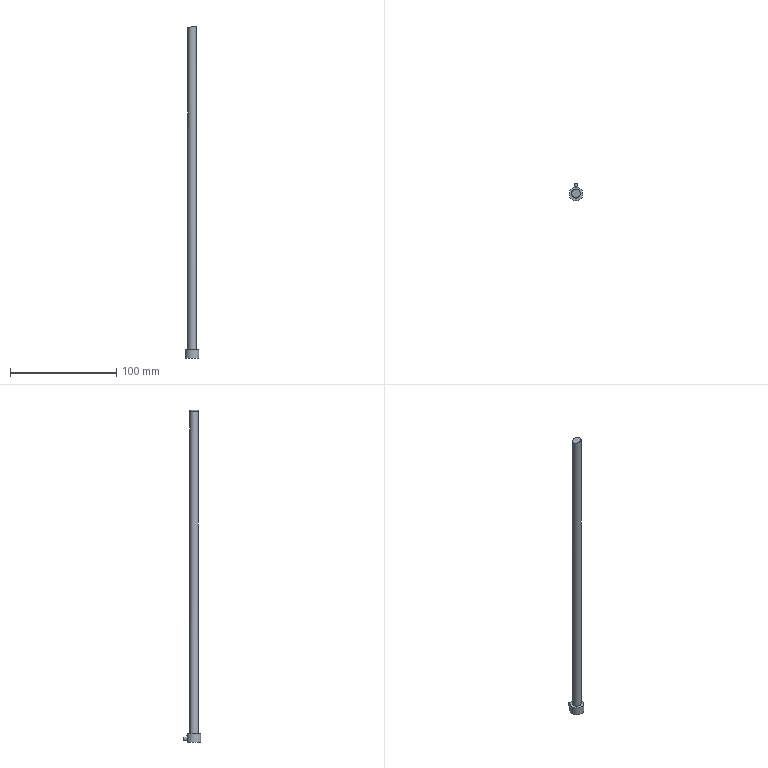Part | STEP file | E108-03-320 | 1 solid | 8 faces | box 13 x 16.5 x 312.703 mm | volume 16360 mm3 | cylinder 3 | plane 3 | spline 1 | cone 1 | commonest cylinder face diameters 3 x1 8 x1 13 x1
STEP:
#1=CARTESIAN_POINT('',(0.,0.,0.));
#2=DIRECTION('',(0.,0.,1.));
#3=DIRECTION('',(1.,0.,0.));
#4=AXIS2_PLACEMENT_3D('',#1,#2,#3);
#5=CARTESIAN_POINT('',(-3.956,0.5934,310.968));
#6=VERTEX_POINT('',#5);
#7=CARTESIAN_POINT('',(-3.956,0.5934,310.968));
#8=CARTESIAN_POINT('',(-4.021,0.1589,310.969));
#9=CARTESIAN_POINT('',(-4.013,-0.2925,310.988));
#10=CARTESIAN_POINT('',(-3.934,-0.7232,311.022));
#11=CARTESIAN_POINT('',(-3.855,-1.154,311.057));
#12=CARTESIAN_POINT('',(-3.702,-1.575,311.108));
#13=CARTESIAN_POINT('',(-3.49,-1.955,311.17));
#14=CARTESIAN_POINT('',(-3.275,-2.338,311.234));
#15=CARTESIAN_POINT('',(-2.993,-2.689,311.311));
#16=CARTESIAN_POINT('',(-2.668,-2.98,311.395));
#17=CARTESIAN_POINT('',(-2.335,-3.279,311.481));
#18=CARTESIAN_POINT('',(-1.947,-3.523,311.576));
#19=CARTESIAN_POINT('',(-1.535,-3.694,311.673));
#20=CARTESIAN_POINT('',(-1.116,-3.868,311.772));
#21=CARTESIAN_POINT('',(-0.6599,-3.971,311.874));
#22=CARTESIAN_POINT('',(-0.2055,-3.995,311.972));
#23=CARTESIAN_POINT('',(0.2524,-4.018,312.071));
#24=CARTESIAN_POINT('',(0.7217,-3.961,312.168));
#25=CARTESIAN_POINT('',(1.163,-3.827,312.255));
#26=CARTESIAN_POINT('',(1.6,-3.694,312.342));
#27=CARTESIAN_POINT('',(2.022,-3.482,312.42));
#28=CARTESIAN_POINT('',(2.391,-3.206,312.485));
#29=CARTESIAN_POINT('',(2.753,-2.936,312.549));
#30=CARTESIAN_POINT('',(3.075,-2.598,312.601));
#31=CARTESIAN_POINT('',(3.328,-2.22,312.637));
#32=CARTESIAN_POINT('',(3.575,-1.849,312.673));
#33=CARTESIAN_POINT('',(3.762,-1.43,312.695));
#34=CARTESIAN_POINT('',(3.874,-0.9979,312.701));
#35=CARTESIAN_POINT('',(3.983,-0.5714,312.707));
#36=CARTESIAN_POINT('',(4.022,-0.1202,312.698));
#37=CARTESIAN_POINT('',(3.987,0.3182,312.675));
#38=CARTESIAN_POINT('',(3.952,0.7555,312.652));
#39=CARTESIAN_POINT('',(3.843,1.192,312.614));
#40=CARTESIAN_POINT('',(3.669,1.593,312.565));
#41=CARTESIAN_POINT('',(3.494,1.997,312.516));
#42=CARTESIAN_POINT('',(3.248,2.375,312.453));
#43=CARTESIAN_POINT('',(2.953,2.698,312.381));
#44=CARTESIAN_POINT('',(2.653,3.027,312.309));
#45=CARTESIAN_POINT('',(2.293,3.307,312.225));
#46=CARTESIAN_POINT('',(1.904,3.518,312.137));
#47=CARTESIAN_POINT('',(1.508,3.732,312.048));
#48=CARTESIAN_POINT('',(1.069,3.881,311.951));
#49=CARTESIAN_POINT('',(0.6254,3.951,311.854));
#50=CARTESIAN_POINT('',(0.1749,4.022,311.757));
#51=CARTESIAN_POINT('',(-0.2942,4.015,311.656));
#52=CARTESIAN_POINT('',(-0.7432,3.93,311.562));
#53=CARTESIAN_POINT('',(-1.193,3.845,311.467));
#54=CARTESIAN_POINT('',(-1.636,3.679,311.376));
#55=CARTESIAN_POINT('',(-2.033,3.445,311.297));
#56=CARTESIAN_POINT('',(-2.425,3.213,311.218));
#57=CARTESIAN_POINT('',(-2.784,2.908,311.149));
#58=CARTESIAN_POINT('',(-3.078,2.555,311.095));
#59=CARTESIAN_POINT('',(-3.364,2.21,311.043));
#60=CARTESIAN_POINT('',(-3.596,1.809,311.005));
#61=CARTESIAN_POINT('',(-3.753,1.385,310.985));
#62=CARTESIAN_POINT('',(-3.847,1.13,310.973));
#63=CARTESIAN_POINT('',(-3.915,0.8629,310.967));
#64=CARTESIAN_POINT('',(-3.956,0.5934,310.968));
#65=B_SPLINE_CURVE_WITH_KNOTS('',3,(#7,#8,#9,#10,#11,#12,#13,#14,#15,#16,#17,#18,#19,#20,#21,#22,#23,#24,#25,#26,#27,#28,#29,#30,#31,#32,#33,#34,#35,#36,#37,#38,#39,#40,#41,#42,#43,#44,#45,#46,#47,#48,#49,#50,#51,#52,#53,#54,#55,#56,#57,#58,#59,#60,#61,#62,#63,#64),.UNSPECIFIED.,.T.,.F.,(1,3,3,3,3,3,3,3,3,3,3,3,3,3,3,3,3,3,3,3,3,1),(-0.03202,0.,0.05208,0.1041,0.1568,0.2108,0.266,0.3216,0.3768,0.431,0.4839,0.5361,0.5882,0.6407,0.6942,0.7487,0.804,0.8595,0.9144,0.968,1.,1.052),.UNSPECIFIED.);
#66=CARTESIAN_POINT('',(0.,0.,108.));
#67=DIRECTION('',(0.,0.,-1.));
#68=DIRECTION('',(-1.,0.,0.));
#69=AXIS2_PLACEMENT_3D('',#66,#67,#68);
#70=CYLINDRICAL_SURFACE('',#69,4.);
#71=CARTESIAN_POINT('',(6.432,-202.968));
#72=CARTESIAN_POINT('',(6.408,-202.968));
#73=CARTESIAN_POINT('',(6.36,-202.971));
#74=CARTESIAN_POINT('',(6.288,-202.979));
#75=CARTESIAN_POINT('',(6.215,-202.992));
#76=CARTESIAN_POINT('',(6.143,-203.009));
#77=CARTESIAN_POINT('',(6.072,-203.031));
#78=CARTESIAN_POINT('',(6.,-203.058));
#79=CARTESIAN_POINT('',(5.928,-203.089));
#80=CARTESIAN_POINT('',(5.856,-203.124));
#81=CARTESIAN_POINT('',(5.784,-203.163));
#82=CARTESIAN_POINT('',(5.713,-203.205));
#83=CARTESIAN_POINT('',(5.642,-203.251));
#84=CARTESIAN_POINT('',(5.57,-203.3));
#85=CARTESIAN_POINT('',(5.499,-203.352));
#86=CARTESIAN_POINT('',(5.428,-203.405));
#87=CARTESIAN_POINT('',(5.358,-203.461));
#88=CARTESIAN_POINT('',(5.287,-203.519));
#89=CARTESIAN_POINT('',(5.216,-203.579));
#90=CARTESIAN_POINT('',(5.145,-203.639));
#91=CARTESIAN_POINT('',(5.075,-203.7));
#92=CARTESIAN_POINT('',(5.004,-203.762));
#93=CARTESIAN_POINT('',(4.934,-203.824));
#94=CARTESIAN_POINT('',(4.863,-203.886));
#95=CARTESIAN_POINT('',(4.792,-203.948));
#96=CARTESIAN_POINT('',(4.722,-204.008));
#97=CARTESIAN_POINT('',(4.651,-204.068));
#98=CARTESIAN_POINT('',(4.581,-204.127));
#99=CARTESIAN_POINT('',(4.51,-204.184));
#100=CARTESIAN_POINT('',(4.439,-204.239));
#101=CARTESIAN_POINT('',(4.368,-204.292));
#102=CARTESIAN_POINT('',(4.297,-204.343));
#103=CARTESIAN_POINT('',(4.226,-204.391));
#104=CARTESIAN_POINT('',(4.154,-204.437));
#105=CARTESIAN_POINT('',(4.083,-204.479));
#106=CARTESIAN_POINT('',(4.012,-204.518));
#107=CARTESIAN_POINT('',(3.94,-204.554));
#108=CARTESIAN_POINT('',(3.868,-204.587));
#109=CARTESIAN_POINT('',(3.796,-204.615));
#110=CARTESIAN_POINT('',(3.724,-204.64));
#111=CARTESIAN_POINT('',(3.653,-204.661));
#112=CARTESIAN_POINT('',(3.58,-204.677));
#113=CARTESIAN_POINT('',(3.508,-204.69));
#114=CARTESIAN_POINT('',(3.436,-204.699));
#115=CARTESIAN_POINT('',(3.364,-204.703));
#116=CARTESIAN_POINT('',(3.292,-204.703));
#117=CARTESIAN_POINT('',(3.219,-204.699));
#118=CARTESIAN_POINT('',(3.147,-204.69));
#119=CARTESIAN_POINT('',(3.075,-204.678));
#120=CARTESIAN_POINT('',(3.003,-204.662));
#121=CARTESIAN_POINT('',(2.931,-204.641));
#122=CARTESIAN_POINT('',(2.859,-204.617));
#123=CARTESIAN_POINT('',(2.787,-204.589));
#124=CARTESIAN_POINT('',(2.715,-204.558));
#125=CARTESIAN_POINT('',(2.643,-204.523));
#126=CARTESIAN_POINT('',(2.572,-204.485));
#127=CARTESIAN_POINT('',(2.5,-204.443));
#128=CARTESIAN_POINT('',(2.429,-204.399));
#129=CARTESIAN_POINT('',(2.358,-204.353));
#130=CARTESIAN_POINT('',(2.286,-204.303));
#131=CARTESIAN_POINT('',(2.215,-204.252));
#132=CARTESIAN_POINT('',(2.144,-204.198));
#133=CARTESIAN_POINT('',(2.073,-204.143));
#134=CARTESIAN_POINT('',(2.003,-204.086));
#135=CARTESIAN_POINT('',(1.932,-204.028));
#136=CARTESIAN_POINT('',(1.861,-203.968));
#137=CARTESIAN_POINT('',(1.79,-203.908));
#138=CARTESIAN_POINT('',(1.72,-203.848));
#139=CARTESIAN_POINT('',(1.649,-203.787));
#140=CARTESIAN_POINT('',(1.579,-203.726));
#141=CARTESIAN_POINT('',(1.508,-203.666));
#142=CARTESIAN_POINT('',(1.437,-203.606));
#143=CARTESIAN_POINT('',(1.367,-203.548));
#144=CARTESIAN_POINT('',(1.296,-203.49));
#145=CARTESIAN_POINT('',(1.225,-203.434));
#146=CARTESIAN_POINT('',(1.154,-203.38));
#147=CARTESIAN_POINT('',(1.083,-203.328));
#148=CARTESIAN_POINT('',(1.012,-203.279));
#149=CARTESIAN_POINT('',(0.941,-203.232));
#150=CARTESIAN_POINT('',(0.8695,-203.188));
#151=CARTESIAN_POINT('',(0.7978,-203.148));
#152=CARTESIAN_POINT('',(0.7262,-203.111));
#153=CARTESIAN_POINT('',(0.6549,-203.077));
#154=CARTESIAN_POINT('',(0.583,-203.048));
#155=CARTESIAN_POINT('',(0.5109,-203.023));
#156=CARTESIAN_POINT('',(0.4386,-203.003));
#157=CARTESIAN_POINT('',(0.3668,-202.987));
#158=CARTESIAN_POINT('',(0.2943,-202.975));
#159=CARTESIAN_POINT('',(0.2215,-202.969));
#160=CARTESIAN_POINT('',(0.1731,-202.968));
#161=CARTESIAN_POINT('',(0.1489,-202.968));
#162=B_SPLINE_CURVE_WITH_KNOTS('',3,(#71,#72,#73,#74,#75,#76,#77,#78,#79,#80,#81,#82,#83,#84,#85,#86,#87,#88,#89,#90,#91,#92,#93,#94,#95,#96,#97,#98,#99,#100,#101,#102,#103,#104,#105,#106,#107,#108,#109,#110,#111,#112,#113,#114,#115,#116,#117,#118,#119,#120,#121,#122,#123,#124,#125,#126,#127,#128,#129,#130,#131,#132,#133,#134,#135,#136,#137,#138,#139,#140,#141,#142,#143,#144,#145,#146,#147,#148,#149,#150,#151,#152,#153,#154,#155,#156,#157,#158,#159,#160,#161),.UNSPECIFIED.,.F.,.F.,(4,1,1,1,1,1,1,1,1,1,1,1,1,1,1,1,1,1,1,1,1,1,1,1,1,1,1,1,1,1,1,1,1,1,1,1,1,1,1,1,1,1,1,1,1,1,1,1,1,1,1,1,1,1,1,1,1,1,1,1,1,1,1,1,1,1,1,1,1,1,1,1,1,1,1,1,1,1,1,1,1,1,1,1,1,1,1,1,4),(0.,0.01136,0.02273,0.03409,0.04545,0.05682,0.06818,0.07955,0.09091,0.1023,0.1136,0.125,0.1364,0.1477,0.1591,0.1705,0.1818,0.1932,0.2045,0.2159,0.2273,0.2386,0.25,0.2614,0.2727,0.2841,0.2955,0.3068,0.3182,0.3295,0.3409,0.3523,0.3636,0.375,0.3864,0.3977,0.4091,0.4205,0.4318,0.4432,0.4545,0.4659,0.4773,0.4886,0.5,0.5114,0.5227,0.5341,0.5455,0.5568,0.5682,0.5795,0.5909,0.6023,0.6136,0.625,0.6364,0.6477,0.6591,0.6705,0.6818,0.6932,0.7045,0.7159,0.7273,0.7386,0.75,0.7614,0.7727,0.7841,0.7955,0.8068,0.8182,0.8295,0.8409,0.8523,0.8636,0.875,0.8864,0.8977,0.9091,0.9205,0.9318,0.9432,0.9545,0.9659,0.9773,0.9886,1.),.QUASI_UNIFORM_KNOTS.);
#163=(GEOMETRIC_REPRESENTATION_CONTEXT(2)PARAMETRIC_REPRESENTATION_CONTEXT()REPRESENTATION_CONTEXT('',''));
#164=DEFINITIONAL_REPRESENTATION('',(#162),#163);
#165=PCURVE('',#70,#164);
#166=CARTESIAN_POINT('',(-4.984,-7.122,311.018));
#167=CARTESIAN_POINT('',(-1.231,-7.119,311.896));
#168=CARTESIAN_POINT('',(2.537,-7.117,312.689));
#169=CARTESIAN_POINT('',(6.321,-7.115,313.394));
#170=CARTESIAN_POINT('',(-4.925,-2.039,310.842));
#171=CARTESIAN_POINT('',(-1.173,-2.037,311.72));
#172=CARTESIAN_POINT('',(2.593,-2.035,312.514));
#173=CARTESIAN_POINT('',(6.376,-2.033,313.219));
#174=CARTESIAN_POINT('',(-4.869,3.043,310.664));
#175=CARTESIAN_POINT('',(-1.118,3.045,311.543));
#176=CARTESIAN_POINT('',(2.646,3.047,312.337));
#177=CARTESIAN_POINT('',(6.428,3.049,313.043));
#178=CARTESIAN_POINT('',(-4.816,8.125,310.485));
#179=CARTESIAN_POINT('',(-1.066,8.127,311.364));
#180=CARTESIAN_POINT('',(2.697,8.129,312.159));
#181=CARTESIAN_POINT('',(6.478,8.131,312.866));
#182=B_SPLINE_SURFACE_WITH_KNOTS('',3,3,((#166,#167,#168,#169),(#170,#171,#172,#173),(#174,#175,#176,#177),(#178,#179,#180,#181)),.UNSPECIFIED.,.F.,.F.,.F.,(4,4),(4,4),(0.,1.),(0.,1.),.PIECEWISE_BEZIER_KNOTS.);
#183=CARTESIAN_POINT('',(0.506,0.0836));
#184=CARTESIAN_POINT('',(0.4998,0.08243));
#185=CARTESIAN_POINT('',(0.4872,0.08071));
#186=CARTESIAN_POINT('',(0.4683,0.07997));
#187=CARTESIAN_POINT('',(0.4493,0.08106));
#188=CARTESIAN_POINT('',(0.4304,0.08398));
#189=CARTESIAN_POINT('',(0.4119,0.0887));
#190=CARTESIAN_POINT('',(0.3936,0.09527));
#191=CARTESIAN_POINT('',(0.3756,0.1036));
#192=CARTESIAN_POINT('',(0.3582,0.1136));
#193=CARTESIAN_POINT('',(0.3414,0.1252));
#194=CARTESIAN_POINT('',(0.3253,0.1383));
#195=CARTESIAN_POINT('',(0.3099,0.153));
#196=CARTESIAN_POINT('',(0.2953,0.1691));
#197=CARTESIAN_POINT('',(0.2816,0.1865));
#198=CARTESIAN_POINT('',(0.2689,0.205));
#199=CARTESIAN_POINT('',(0.2572,0.2248));
#200=CARTESIAN_POINT('',(0.2465,0.2456));
#201=CARTESIAN_POINT('',(0.237,0.2673));
#202=CARTESIAN_POINT('',(0.2286,0.2898));
#203=CARTESIAN_POINT('',(0.2214,0.3128));
#204=CARTESIAN_POINT('',(0.2155,0.3366));
#205=CARTESIAN_POINT('',(0.2108,0.3609));
#206=CARTESIAN_POINT('',(0.2073,0.3856));
#207=CARTESIAN_POINT('',(0.2052,0.4105));
#208=CARTESIAN_POINT('',(0.2043,0.4353));
#209=CARTESIAN_POINT('',(0.2048,0.4604));
#210=CARTESIAN_POINT('',(0.2066,0.4853));
#211=CARTESIAN_POINT('',(0.2097,0.5101));
#212=CARTESIAN_POINT('',(0.214,0.5344));
#213=CARTESIAN_POINT('',(0.2197,0.5581));
#214=CARTESIAN_POINT('',(0.2266,0.5814));
#215=CARTESIAN_POINT('',(0.2348,0.604));
#216=CARTESIAN_POINT('',(0.2441,0.6257));
#217=CARTESIAN_POINT('',(0.2545,0.6465));
#218=CARTESIAN_POINT('',(0.2661,0.6661));
#219=CARTESIAN_POINT('',(0.2787,0.6847));
#220=CARTESIAN_POINT('',(0.2924,0.7021));
#221=CARTESIAN_POINT('',(0.3069,0.7181));
#222=CARTESIAN_POINT('',(0.3222,0.7326));
#223=CARTESIAN_POINT('',(0.3384,0.7456));
#224=CARTESIAN_POINT('',(0.3552,0.757));
#225=CARTESIAN_POINT('',(0.3727,0.7668));
#226=CARTESIAN_POINT('',(0.3906,0.7748));
#227=CARTESIAN_POINT('',(0.4089,0.7811));
#228=CARTESIAN_POINT('',(0.4275,0.7855));
#229=CARTESIAN_POINT('',(0.4464,0.7881));
#230=CARTESIAN_POINT('',(0.4654,0.7889));
#231=CARTESIAN_POINT('',(0.4843,0.7879));
#232=CARTESIAN_POINT('',(0.503,0.785));
#233=CARTESIAN_POINT('',(0.5217,0.7803));
#234=CARTESIAN_POINT('',(0.5401,0.7738));
#235=CARTESIAN_POINT('',(0.558,0.7656));
#236=CARTESIAN_POINT('',(0.5754,0.7557));
#237=CARTESIAN_POINT('',(0.5922,0.7442));
#238=CARTESIAN_POINT('',(0.6084,0.731));
#239=CARTESIAN_POINT('',(0.6239,0.7164));
#240=CARTESIAN_POINT('',(0.6386,0.7004));
#241=CARTESIAN_POINT('',(0.6522,0.6831));
#242=CARTESIAN_POINT('',(0.665,0.6645));
#243=CARTESIAN_POINT('',(0.6767,0.6447));
#244=CARTESIAN_POINT('',(0.6874,0.6239));
#245=CARTESIAN_POINT('',(0.697,0.6023));
#246=CARTESIAN_POINT('',(0.7053,0.5799));
#247=CARTESIAN_POINT('',(0.7125,0.5566));
#248=CARTESIAN_POINT('',(0.7184,0.5328));
#249=CARTESIAN_POINT('',(0.7232,0.5084));
#250=CARTESIAN_POINT('',(0.7266,0.4839));
#251=CARTESIAN_POINT('',(0.7287,0.459));
#252=CARTESIAN_POINT('',(0.7295,0.434));
#253=CARTESIAN_POINT('',(0.729,0.4089));
#254=CARTESIAN_POINT('',(0.7272,0.384));
#255=CARTESIAN_POINT('',(0.7241,0.3594));
#256=CARTESIAN_POINT('',(0.7197,0.3351));
#257=CARTESIAN_POINT('',(0.714,0.3112));
#258=CARTESIAN_POINT('',(0.7071,0.2879));
#259=CARTESIAN_POINT('',(0.6989,0.2653));
#260=CARTESIAN_POINT('',(0.6897,0.2437));
#261=CARTESIAN_POINT('',(0.6792,0.2229));
#262=CARTESIAN_POINT('',(0.6676,0.2031));
#263=CARTESIAN_POINT('',(0.655,0.1844));
#264=CARTESIAN_POINT('',(0.6414,0.167));
#265=CARTESIAN_POINT('',(0.627,0.1511));
#266=CARTESIAN_POINT('',(0.6116,0.1365));
#267=CARTESIAN_POINT('',(0.5954,0.1235));
#268=CARTESIAN_POINT('',(0.5786,0.112));
#269=CARTESIAN_POINT('',(0.5612,0.1022));
#270=CARTESIAN_POINT('',(0.5432,0.09409));
#271=CARTESIAN_POINT('',(0.5248,0.08777));
#272=CARTESIAN_POINT('',(0.5123,0.08478));
#273=CARTESIAN_POINT('',(0.506,0.0836));
#274=B_SPLINE_CURVE_WITH_KNOTS('',3,(#183,#184,#185,#186,#187,#188,#189,#190,#191,#192,#193,#194,#195,#196,#197,#198,#199,#200,#201,#202,#203,#204,#205,#206,#207,#208,#209,#210,#211,#212,#213,#214,#215,#216,#217,#218,#219,#220,#221,#222,#223,#224,#225,#226,#227,#228,#229,#230,#231,#232,#233,#234,#235,#236,#237,#238,#239,#240,#241,#242,#243,#244,#245,#246,#247,#248,#249,#250,#251,#252,#253,#254,#255,#256,#257,#258,#259,#260,#261,#262,#263,#264,#265,#266,#267,#268,#269,#270,#271,#272,#273),.UNSPECIFIED.,.T.,.F.,(4,1,1,1,1,1,1,1,1,1,1,1,1,1,1,1,1,1,1,1,1,1,1,1,1,1,1,1,1,1,1,1,1,1,1,1,1,1,1,1,1,1,1,1,1,1,1,1,1,1,1,1,1,1,1,1,1,1,1,1,1,1,1,1,1,1,1,1,1,1,1,1,1,1,1,1,1,1,1,1,1,1,1,1,1,1,1,1,4),(0.,0.01136,0.02273,0.03409,0.04545,0.05682,0.06818,0.07955,0.09091,0.1023,0.1136,0.125,0.1364,0.1477,0.1591,0.1705,0.1818,0.1932,0.2045,0.2159,0.2273,0.2386,0.25,0.2614,0.2727,0.2841,0.2955,0.3068,0.3182,0.3295,0.3409,0.3523,0.3636,0.375,0.3864,0.3977,0.4091,0.4205,0.4318,0.4432,0.4545,0.4659,0.4773,0.4886,0.5,0.5114,0.5227,0.5341,0.5455,0.5568,0.5682,0.5795,0.5909,0.6023,0.6136,0.625,0.6364,0.6477,0.6591,0.6705,0.6818,0.6932,0.7045,0.7159,0.7273,0.7386,0.75,0.7614,0.7727,0.7841,0.7955,0.8068,0.8182,0.8295,0.8409,0.8523,0.8636,0.875,0.8864,0.8977,0.9091,0.9205,0.9318,0.9432,0.9545,0.9659,0.9773,0.9886,1.),.QUASI_UNIFORM_KNOTS.);
#275=(GEOMETRIC_REPRESENTATION_CONTEXT(2)PARAMETRIC_REPRESENTATION_CONTEXT()REPRESENTATION_CONTEXT('',''));
#276=DEFINITIONAL_REPRESENTATION('',(#274),#275);
#277=PCURVE('',#182,#276);
#278=SURFACE_CURVE('',#65,(#165,#277),.PCURVE_S1.);
#279=EDGE_CURVE('',#6,#6,#278,.T.);
#280=ORIENTED_EDGE('',*,*,#279,.F.);
#281=CARTESIAN_POINT('',(-3.956,0.5934,8.));
#282=VERTEX_POINT('',#281);
#283=CARTESIAN_POINT('',(-3.956,0.5934,310.968));
#284=CARTESIAN_POINT('',(-3.956,0.5934,8.));
#285=B_SPLINE_CURVE_WITH_KNOTS('',1,(#283,#284),.UNSPECIFIED.,.F.,.F.,(2,2),(-202.968,100.),.PIECEWISE_BEZIER_KNOTS.);
#286=CARTESIAN_POINT('',(6.432,0.));
#287=DIRECTION('',(0.,1.));
#288=VECTOR('',#287,1.);
#289=LINE('',#286,#288);
#290=(GEOMETRIC_REPRESENTATION_CONTEXT(2)PARAMETRIC_REPRESENTATION_CONTEXT()REPRESENTATION_CONTEXT('',''));
#291=DEFINITIONAL_REPRESENTATION('',(#289),#290);
#292=PCURVE('',#70,#291);
#293=CARTESIAN_POINT('',(0.1489,0.));
#294=DIRECTION('',(0.,1.));
#295=VECTOR('',#294,1.);
#296=LINE('',#293,#295);
#297=(GEOMETRIC_REPRESENTATION_CONTEXT(2)PARAMETRIC_REPRESENTATION_CONTEXT()REPRESENTATION_CONTEXT('',''));
#298=DEFINITIONAL_REPRESENTATION('',(#296),#297);
#299=PCURVE('',#70,#298);
#300=SEAM_CURVE('',#285,(#292,#299),.PCURVE_S1.);
#301=EDGE_CURVE('',#6,#282,#300,.T.);
#302=ORIENTED_EDGE('',*,*,#301,.T.);
#303=CARTESIAN_POINT('',(4.,0.,8.));
#304=VERTEX_POINT('',#303);
#305=CARTESIAN_POINT('',(0.,0.,8.));
#306=DIRECTION('',(0.,0.,1.));
#307=DIRECTION('',(1.,0.,0.));
#308=AXIS2_PLACEMENT_3D('',#305,#306,#307);
#309=CIRCLE('',#308,4.);
#310=CARTESIAN_POINT('',(9.425,100.));
#311=DIRECTION('',(-1.,0.));
#312=VECTOR('',#311,1.);
#313=LINE('',#310,#312);
#314=(GEOMETRIC_REPRESENTATION_CONTEXT(2)PARAMETRIC_REPRESENTATION_CONTEXT()REPRESENTATION_CONTEXT('',''));
#315=DEFINITIONAL_REPRESENTATION('',(#313),#314);
#316=PCURVE('',#70,#315);
#317=CARTESIAN_POINT('',(0.,0.,8.));
#318=DIRECTION('',(0.,0.,-1.));
#319=DIRECTION('',(1.,0.,0.));
#320=AXIS2_PLACEMENT_3D('',#317,#318,#319);
#321=PLANE('',#320);
#322=CARTESIAN_POINT('',(4.,0.));
#323=CARTESIAN_POINT('',(4.,-6.928));
#324=CARTESIAN_POINT('',(-2.,-3.464));
#325=CARTESIAN_POINT('',(-8.,0.));
#326=CARTESIAN_POINT('',(-2.,3.464));
#327=CARTESIAN_POINT('',(4.,6.928));
#328=CARTESIAN_POINT('',(4.,0.));
#329=(BOUNDED_CURVE()B_SPLINE_CURVE(2,(#322,#323,#324,#325,#326,#327,#328),.UNSPECIFIED.,.T.,.F.)B_SPLINE_CURVE_WITH_KNOTS((1,2,2,2,2,1),(-2.094,0.,2.094,4.189,6.283,8.378),.UNSPECIFIED.)CURVE()GEOMETRIC_REPRESENTATION_ITEM()RATIONAL_B_SPLINE_CURVE((1.,0.5,1.,0.5,1.,0.5,1.))REPRESENTATION_ITEM(''));
#330=(GEOMETRIC_REPRESENTATION_CONTEXT(2)PARAMETRIC_REPRESENTATION_CONTEXT()REPRESENTATION_CONTEXT('',''));
#331=DEFINITIONAL_REPRESENTATION('',(#329),#330);
#332=PCURVE('',#321,#331);
#333=SURFACE_CURVE('',#309,(#316,#332),.PCURVE_S1.);
#334=EDGE_CURVE('',#282,#304,#333,.T.);
#335=ORIENTED_EDGE('',*,*,#334,.T.);
#336=CARTESIAN_POINT('',(0.,0.,8.));
#337=DIRECTION('',(0.,0.,1.));
#338=DIRECTION('',(1.,0.,0.));
#339=AXIS2_PLACEMENT_3D('',#336,#337,#338);
#340=CIRCLE('',#339,4.);
#341=CARTESIAN_POINT('',(3.142,100.));
#342=DIRECTION('',(-1.,0.));
#343=VECTOR('',#342,1.);
#344=LINE('',#341,#343);
#345=(GEOMETRIC_REPRESENTATION_CONTEXT(2)PARAMETRIC_REPRESENTATION_CONTEXT()REPRESENTATION_CONTEXT('',''));
#346=DEFINITIONAL_REPRESENTATION('',(#344),#345);
#347=PCURVE('',#70,#346);
#348=CARTESIAN_POINT('',(4.,0.));
#349=CARTESIAN_POINT('',(4.,-6.928));
#350=CARTESIAN_POINT('',(-2.,-3.464));
#351=CARTESIAN_POINT('',(-8.,0.));
#352=CARTESIAN_POINT('',(-2.,3.464));
#353=CARTESIAN_POINT('',(4.,6.928));
#354=CARTESIAN_POINT('',(4.,0.));
#355=(BOUNDED_CURVE()B_SPLINE_CURVE(2,(#348,#349,#350,#351,#352,#353,#354),.UNSPECIFIED.,.T.,.F.)B_SPLINE_CURVE_WITH_KNOTS((1,2,2,2,2,1),(-2.094,0.,2.094,4.189,6.283,8.378),.UNSPECIFIED.)CURVE()GEOMETRIC_REPRESENTATION_ITEM()RATIONAL_B_SPLINE_CURVE((1.,0.5,1.,0.5,1.,0.5,1.))REPRESENTATION_ITEM(''));
#356=(GEOMETRIC_REPRESENTATION_CONTEXT(2)PARAMETRIC_REPRESENTATION_CONTEXT()REPRESENTATION_CONTEXT('',''));
#357=DEFINITIONAL_REPRESENTATION('',(#355),#356);
#358=PCURVE('',#321,#357);
#359=SURFACE_CURVE('',#340,(#347,#358),.PCURVE_S1.);
#360=EDGE_CURVE('',#304,#282,#359,.T.);
#361=ORIENTED_EDGE('',*,*,#360,.T.);
#362=ORIENTED_EDGE('',*,*,#301,.F.);
#363=EDGE_LOOP('',(#280,#302,#335,#361,#362));
#364=FACE_BOUND('',#363,.T.);
#365=ADVANCED_FACE('',(#364),#70,.T.);
#366=ORIENTED_EDGE('',*,*,#279,.F.);
#367=EDGE_LOOP('',(#366));
#368=FACE_BOUND('',#367,.F.);
#369=ADVANCED_FACE('',(#368),#182,.F.);
#370=CARTESIAN_POINT('',(6.5,0.,0.));
#371=VERTEX_POINT('',#370);
#372=CARTESIAN_POINT('',(-6.5,0.,0.));
#373=VERTEX_POINT('',#372);
#374=CARTESIAN_POINT('',(0.,0.,0.));
#375=DIRECTION('',(0.,0.,-1.));
#376=DIRECTION('',(-1.,0.,0.));
#377=AXIS2_PLACEMENT_3D('',#374,#375,#376);
#378=CIRCLE('',#377,6.5);
#379=CARTESIAN_POINT('',(0.,0.,8.));
#380=DIRECTION('',(0.,0.,-1.));
#381=DIRECTION('',(1.,0.,0.));
#382=AXIS2_PLACEMENT_3D('',#379,#380,#381);
#383=CYLINDRICAL_SURFACE('',#382,6.5);
#384=CARTESIAN_POINT('',(-3.142,8.));
#385=DIRECTION('',(1.,0.));
#386=VECTOR('',#385,1.);
#387=LINE('',#384,#386);
#388=(GEOMETRIC_REPRESENTATION_CONTEXT(2)PARAMETRIC_REPRESENTATION_CONTEXT()REPRESENTATION_CONTEXT('',''));
#389=DEFINITIONAL_REPRESENTATION('',(#387),#388);
#390=PCURVE('',#383,#389);
#391=CARTESIAN_POINT('',(240.,-1000.,0.));
#392=DIRECTION('',(0.,0.,1.));
#393=DIRECTION('',(-1.,0.,0.));
#394=AXIS2_PLACEMENT_3D('',#391,#392,#393);
#395=PLANE('',#394);
#396=CARTESIAN_POINT('',(246.5,-1000.));
#397=CARTESIAN_POINT('',(246.5,-1011.258));
#398=CARTESIAN_POINT('',(236.75,-1005.629));
#399=CARTESIAN_POINT('',(227.,-1000.));
#400=CARTESIAN_POINT('',(236.75,-994.371));
#401=CARTESIAN_POINT('',(246.5,-988.742));
#402=CARTESIAN_POINT('',(246.5,-1000.));
#403=(BOUNDED_CURVE()B_SPLINE_CURVE(2,(#396,#397,#398,#399,#400,#401,#402),.UNSPECIFIED.,.T.,.F.)B_SPLINE_CURVE_WITH_KNOTS((1,2,2,2,2,1),(-2.094,0.,2.094,4.189,6.283,8.378),.UNSPECIFIED.)CURVE()GEOMETRIC_REPRESENTATION_ITEM()RATIONAL_B_SPLINE_CURVE((1.,0.5,1.,0.5,1.,0.5,1.))REPRESENTATION_ITEM(''));
#404=(GEOMETRIC_REPRESENTATION_CONTEXT(2)PARAMETRIC_REPRESENTATION_CONTEXT()REPRESENTATION_CONTEXT('',''));
#405=DEFINITIONAL_REPRESENTATION('',(#403),#404);
#406=PCURVE('',#395,#405);
#407=SURFACE_CURVE('',#378,(#390,#406),.PCURVE_S1.);
#408=EDGE_CURVE('',#371,#373,#407,.T.);
#409=ORIENTED_EDGE('',*,*,#408,.F.);
#410=CARTESIAN_POINT('',(6.5,0.,8.));
#411=VERTEX_POINT('',#410);
#412=CARTESIAN_POINT('',(6.5,0.,8.));
#413=CARTESIAN_POINT('',(6.5,0.,0.));
#414=B_SPLINE_CURVE_WITH_KNOTS('',1,(#412,#413),.UNSPECIFIED.,.F.,.F.,(2,2),(0.,8.),.PIECEWISE_BEZIER_KNOTS.);
#415=CARTESIAN_POINT('',(0.,0.));
#416=DIRECTION('',(0.,1.));
#417=VECTOR('',#416,1.);
#418=LINE('',#415,#417);
#419=(GEOMETRIC_REPRESENTATION_CONTEXT(2)PARAMETRIC_REPRESENTATION_CONTEXT()REPRESENTATION_CONTEXT('',''));
#420=DEFINITIONAL_REPRESENTATION('',(#418),#419);
#421=PCURVE('',#383,#420);
#422=CARTESIAN_POINT('',(6.283,0.));
#423=DIRECTION('',(0.,1.));
#424=VECTOR('',#423,1.);
#425=LINE('',#422,#424);
#426=(GEOMETRIC_REPRESENTATION_CONTEXT(2)PARAMETRIC_REPRESENTATION_CONTEXT()REPRESENTATION_CONTEXT('',''));
#427=DEFINITIONAL_REPRESENTATION('',(#425),#426);
#428=PCURVE('',#383,#427);
#429=SEAM_CURVE('',#414,(#421,#428),.PCURVE_S1.);
#430=EDGE_CURVE('',#411,#371,#429,.T.);
#431=ORIENTED_EDGE('',*,*,#430,.F.);
#432=CARTESIAN_POINT('',(0.,0.,8.));
#433=DIRECTION('',(0.,0.,-1.));
#434=DIRECTION('',(1.,0.,0.));
#435=AXIS2_PLACEMENT_3D('',#432,#433,#434);
#436=CIRCLE('',#435,6.5);
#437=CARTESIAN_POINT('',(0.,0.));
#438=DIRECTION('',(1.,0.));
#439=VECTOR('',#438,1.);
#440=LINE('',#437,#439);
#441=(GEOMETRIC_REPRESENTATION_CONTEXT(2)PARAMETRIC_REPRESENTATION_CONTEXT()REPRESENTATION_CONTEXT('',''));
#442=DEFINITIONAL_REPRESENTATION('',(#440),#441);
#443=PCURVE('',#383,#442);
#444=CARTESIAN_POINT('',(0.,0.));
#445=DIRECTION('',(1.,0.));
#446=AXIS2_PLACEMENT_2D('',#444,#445);
#447=CIRCLE('',#446,6.5);
#448=(GEOMETRIC_REPRESENTATION_CONTEXT(2)PARAMETRIC_REPRESENTATION_CONTEXT()REPRESENTATION_CONTEXT('',''));
#449=DEFINITIONAL_REPRESENTATION('',(#447),#448);
#450=PCURVE('',#321,#449);
#451=SURFACE_CURVE('',#436,(#443,#450),.PCURVE_S1.);
#452=EDGE_CURVE('',#411,#411,#451,.T.);
#453=ORIENTED_EDGE('',*,*,#452,.T.);
#454=ORIENTED_EDGE('',*,*,#430,.T.);
#455=CARTESIAN_POINT('',(0.,0.,0.));
#456=DIRECTION('',(0.,0.,-1.));
#457=DIRECTION('',(-1.,0.,0.));
#458=AXIS2_PLACEMENT_3D('',#455,#456,#457);
#459=CIRCLE('',#458,6.5);
#460=CARTESIAN_POINT('',(3.142,8.));
#461=DIRECTION('',(1.,0.));
#462=VECTOR('',#461,1.);
#463=LINE('',#460,#462);
#464=(GEOMETRIC_REPRESENTATION_CONTEXT(2)PARAMETRIC_REPRESENTATION_CONTEXT()REPRESENTATION_CONTEXT('',''));
#465=DEFINITIONAL_REPRESENTATION('',(#463),#464);
#466=PCURVE('',#383,#465);
#467=CARTESIAN_POINT('',(246.5,-1000.));
#468=CARTESIAN_POINT('',(246.5,-1011.258));
#469=CARTESIAN_POINT('',(236.75,-1005.629));
#470=CARTESIAN_POINT('',(227.,-1000.));
#471=CARTESIAN_POINT('',(236.75,-994.371));
#472=CARTESIAN_POINT('',(246.5,-988.742));
#473=CARTESIAN_POINT('',(246.5,-1000.));
#474=(BOUNDED_CURVE()B_SPLINE_CURVE(2,(#467,#468,#469,#470,#471,#472,#473),.UNSPECIFIED.,.T.,.F.)B_SPLINE_CURVE_WITH_KNOTS((1,2,2,2,2,1),(-2.094,0.,2.094,4.189,6.283,8.378),.UNSPECIFIED.)CURVE()GEOMETRIC_REPRESENTATION_ITEM()RATIONAL_B_SPLINE_CURVE((1.,0.5,1.,0.5,1.,0.5,1.))REPRESENTATION_ITEM(''));
#475=(GEOMETRIC_REPRESENTATION_CONTEXT(2)PARAMETRIC_REPRESENTATION_CONTEXT()REPRESENTATION_CONTEXT('',''));
#476=DEFINITIONAL_REPRESENTATION('',(#474),#475);
#477=PCURVE('',#395,#476);
#478=SURFACE_CURVE('',#459,(#466,#477),.PCURVE_S1.);
#479=EDGE_CURVE('',#373,#371,#478,.T.);
#480=ORIENTED_EDGE('',*,*,#479,.F.);
#481=EDGE_LOOP('',(#409,#431,#453,#454,#480));
#482=FACE_BOUND('',#481,.T.);
#483=CARTESIAN_POINT('',(0.,6.5,1.5));
#484=VERTEX_POINT('',#483);
#485=CARTESIAN_POINT('',(0.,6.5,1.5));
#486=CARTESIAN_POINT('',(0.1654,6.5,1.5));
#487=CARTESIAN_POINT('',(0.3332,6.493,1.528));
#488=CARTESIAN_POINT('',(0.4892,6.482,1.582));
#489=CARTESIAN_POINT('',(0.6451,6.47,1.636));
#490=CARTESIAN_POINT('',(0.7936,6.453,1.717));
#491=CARTESIAN_POINT('',(0.9231,6.434,1.818));
#492=CARTESIAN_POINT('',(1.055,6.415,1.92));
#493=CARTESIAN_POINT('',(1.17,6.394,2.047));
#494=CARTESIAN_POINT('',(1.261,6.377,2.187));
#495=CARTESIAN_POINT('',(1.352,6.358,2.329));
#496=CARTESIAN_POINT('',(1.421,6.343,2.49));
#497=CARTESIAN_POINT('',(1.46,6.334,2.655));
#498=CARTESIAN_POINT('',(1.498,6.325,2.817));
#499=CARTESIAN_POINT('',(1.509,6.322,2.989));
#500=CARTESIAN_POINT('',(1.492,6.326,3.155));
#501=CARTESIAN_POINT('',(1.475,6.33,3.318));
#502=CARTESIAN_POINT('',(1.431,6.341,3.48));
#503=CARTESIAN_POINT('',(1.362,6.356,3.628));
#504=CARTESIAN_POINT('',(1.293,6.37,3.777));
#505=CARTESIAN_POINT('',(1.199,6.39,3.917));
#506=CARTESIAN_POINT('',(1.085,6.409,4.035));
#507=CARTESIAN_POINT('',(0.9695,6.428,4.157));
#508=CARTESIAN_POINT('',(0.8309,6.448,4.26));
#509=CARTESIAN_POINT('',(0.6809,6.464,4.337));
#510=CARTESIAN_POINT('',(0.5305,6.48,4.413));
#511=CARTESIAN_POINT('',(0.3642,6.492,4.465));
#512=CARTESIAN_POINT('',(0.1962,6.497,4.487));
#513=CARTESIAN_POINT('',(0.03191,6.502,4.509));
#514=CARTESIAN_POINT('',(-0.1386,6.501,4.503));
#515=CARTESIAN_POINT('',(-0.3008,6.493,4.47));
#516=CARTESIAN_POINT('',(-0.4611,6.486,4.437));
#517=CARTESIAN_POINT('',(-0.6177,6.472,4.377));
#518=CARTESIAN_POINT('',(-0.7583,6.456,4.294));
#519=CARTESIAN_POINT('',(-0.9011,6.439,4.211));
#520=CARTESIAN_POINT('',(-1.031,6.419,4.102));
#521=CARTESIAN_POINT('',(-1.139,6.399,3.976));
#522=CARTESIAN_POINT('',(-1.249,6.38,3.848));
#523=CARTESIAN_POINT('',(-1.338,6.361,3.699));
#524=CARTESIAN_POINT('',(-1.399,6.348,3.541));
#525=CARTESIAN_POINT('',(-1.46,6.334,3.384));
#526=CARTESIAN_POINT('',(-1.494,6.326,3.214));
#527=CARTESIAN_POINT('',(-1.499,6.325,3.046));
#528=CARTESIAN_POINT('',(-1.504,6.324,2.881));
#529=CARTESIAN_POINT('',(-1.482,6.329,2.714));
#530=CARTESIAN_POINT('',(-1.433,6.34,2.557));
#531=CARTESIAN_POINT('',(-1.385,6.351,2.4));
#532=CARTESIAN_POINT('',(-1.309,6.367,2.25));
#533=CARTESIAN_POINT('',(-1.214,6.386,2.119));
#534=CARTESIAN_POINT('',(-1.116,6.404,1.984));
#535=CARTESIAN_POINT('',(-0.9937,6.425,1.864));
#536=CARTESIAN_POINT('',(-0.8569,6.443,1.769));
#537=CARTESIAN_POINT('',(-0.7182,6.462,1.672));
#538=CARTESIAN_POINT('',(-0.5604,6.478,1.598));
#539=CARTESIAN_POINT('',(-0.3967,6.488,1.553));
#540=CARTESIAN_POINT('',(-0.2682,6.496,1.518));
#541=CARTESIAN_POINT('',(-0.1335,6.5,1.5));
#542=CARTESIAN_POINT('',(0.,6.5,1.5));
#543=B_SPLINE_CURVE_WITH_KNOTS('',3,(#485,#486,#487,#488,#489,#490,#491,#492,#493,#494,#495,#496,#497,#498,#499,#500,#501,#502,#503,#504,#505,#506,#507,#508,#509,#510,#511,#512,#513,#514,#515,#516,#517,#518,#519,#520,#521,#522,#523,#524,#525,#526,#527,#528,#529,#530,#531,#532,#533,#534,#535,#536,#537,#538,#539,#540,#541,#542),.UNSPECIFIED.,.T.,.F.,(1,3,3,3,3,3,3,3,3,3,3,3,3,3,3,3,3,3,3,3,3,1),(-0.04234,0.,0.05275,0.1054,0.159,0.2132,0.2665,0.3187,0.3713,0.4252,0.4793,0.5321,0.5843,0.6373,0.6915,0.7453,0.7978,0.85,0.9034,0.9577,1.,1.053),.UNSPECIFIED.);
#544=CARTESIAN_POINT('',(4.712,6.5));
#545=CARTESIAN_POINT('',(4.718,6.5));
#546=CARTESIAN_POINT('',(4.729,6.497));
#547=CARTESIAN_POINT('',(4.745,6.486));
#548=CARTESIAN_POINT('',(4.762,6.467));
#549=CARTESIAN_POINT('',(4.778,6.44));
#550=CARTESIAN_POINT('',(4.793,6.406));
#551=CARTESIAN_POINT('',(4.809,6.365));
#552=CARTESIAN_POINT('',(4.823,6.317));
#553=CARTESIAN_POINT('',(4.838,6.262));
#554=CARTESIAN_POINT('',(4.851,6.201));
#555=CARTESIAN_POINT('',(4.864,6.135));
#556=CARTESIAN_POINT('',(4.876,6.062));
#557=CARTESIAN_POINT('',(4.888,5.983));
#558=CARTESIAN_POINT('',(4.898,5.9));
#559=CARTESIAN_POINT('',(4.908,5.813));
#560=CARTESIAN_POINT('',(4.916,5.721));
#561=CARTESIAN_POINT('',(4.924,5.625));
#562=CARTESIAN_POINT('',(4.93,5.526));
#563=CARTESIAN_POINT('',(4.936,5.424));
#564=CARTESIAN_POINT('',(4.94,5.321));
#565=CARTESIAN_POINT('',(4.943,5.215));
#566=CARTESIAN_POINT('',(4.945,5.108));
#567=CARTESIAN_POINT('',(4.945,5.));
#568=CARTESIAN_POINT('',(4.945,4.893));
#569=CARTESIAN_POINT('',(4.943,4.787));
#570=CARTESIAN_POINT('',(4.94,4.681));
#571=CARTESIAN_POINT('',(4.936,4.576));
#572=CARTESIAN_POINT('',(4.93,4.474));
#573=CARTESIAN_POINT('',(4.924,4.376));
#574=CARTESIAN_POINT('',(4.916,4.28));
#575=CARTESIAN_POINT('',(4.908,4.188));
#576=CARTESIAN_POINT('',(4.898,4.1));
#577=CARTESIAN_POINT('',(4.888,4.017));
#578=CARTESIAN_POINT('',(4.877,3.939));
#579=CARTESIAN_POINT('',(4.864,3.866));
#580=CARTESIAN_POINT('',(4.851,3.799));
#581=CARTESIAN_POINT('',(4.838,3.738));
#582=CARTESIAN_POINT('',(4.824,3.683));
#583=CARTESIAN_POINT('',(4.809,3.635));
#584=CARTESIAN_POINT('',(4.793,3.594));
#585=CARTESIAN_POINT('',(4.778,3.56));
#586=CARTESIAN_POINT('',(4.762,3.533));
#587=CARTESIAN_POINT('',(4.745,3.514));
#588=CARTESIAN_POINT('',(4.729,3.503));
#589=CARTESIAN_POINT('',(4.713,3.499));
#590=CARTESIAN_POINT('',(4.696,3.503));
#591=CARTESIAN_POINT('',(4.679,3.514));
#592=CARTESIAN_POINT('',(4.663,3.533));
#593=CARTESIAN_POINT('',(4.647,3.56));
#594=CARTESIAN_POINT('',(4.632,3.594));
#595=CARTESIAN_POINT('',(4.616,3.635));
#596=CARTESIAN_POINT('',(4.601,3.683));
#597=CARTESIAN_POINT('',(4.587,3.737));
#598=CARTESIAN_POINT('',(4.574,3.798));
#599=CARTESIAN_POINT('',(4.561,3.865));
#600=CARTESIAN_POINT('',(4.548,3.938));
#601=CARTESIAN_POINT('',(4.537,4.016));
#602=CARTESIAN_POINT('',(4.527,4.099));
#603=CARTESIAN_POINT('',(4.517,4.187));
#604=CARTESIAN_POINT('',(4.508,4.279));
#605=CARTESIAN_POINT('',(4.501,4.375));
#606=CARTESIAN_POINT('',(4.494,4.473));
#607=CARTESIAN_POINT('',(4.489,4.575));
#608=CARTESIAN_POINT('',(4.485,4.679));
#609=CARTESIAN_POINT('',(4.482,4.785));
#610=CARTESIAN_POINT('',(4.48,4.892));
#611=CARTESIAN_POINT('',(4.479,4.999));
#612=CARTESIAN_POINT('',(4.48,5.106));
#613=CARTESIAN_POINT('',(4.482,5.213));
#614=CARTESIAN_POINT('',(4.485,5.319));
#615=CARTESIAN_POINT('',(4.489,5.423));
#616=CARTESIAN_POINT('',(4.494,5.524));
#617=CARTESIAN_POINT('',(4.501,5.624));
#618=CARTESIAN_POINT('',(4.508,5.72));
#619=CARTESIAN_POINT('',(4.517,5.812));
#620=CARTESIAN_POINT('',(4.526,5.899));
#621=CARTESIAN_POINT('',(4.537,5.982));
#622=CARTESIAN_POINT('',(4.548,6.061));
#623=CARTESIAN_POINT('',(4.56,6.134));
#624=CARTESIAN_POINT('',(4.573,6.201));
#625=CARTESIAN_POINT('',(4.587,6.262));
#626=CARTESIAN_POINT('',(4.601,6.316));
#627=CARTESIAN_POINT('',(4.616,6.364));
#628=CARTESIAN_POINT('',(4.631,6.406));
#629=CARTESIAN_POINT('',(4.647,6.44));
#630=CARTESIAN_POINT('',(4.663,6.466));
#631=CARTESIAN_POINT('',(4.679,6.486));
#632=CARTESIAN_POINT('',(4.696,6.497));
#633=CARTESIAN_POINT('',(4.707,6.5));
#634=CARTESIAN_POINT('',(4.712,6.5));
#635=B_SPLINE_CURVE_WITH_KNOTS('',3,(#544,#545,#546,#547,#548,#549,#550,#551,#552,#553,#554,#555,#556,#557,#558,#559,#560,#561,#562,#563,#564,#565,#566,#567,#568,#569,#570,#571,#572,#573,#574,#575,#576,#577,#578,#579,#580,#581,#582,#583,#584,#585,#586,#587,#588,#589,#590,#591,#592,#593,#594,#595,#596,#597,#598,#599,#600,#601,#602,#603,#604,#605,#606,#607,#608,#609,#610,#611,#612,#613,#614,#615,#616,#617,#618,#619,#620,#621,#622,#623,#624,#625,#626,#627,#628,#629,#630,#631,#632,#633,#634),.UNSPECIFIED.,.T.,.F.,(4,1,1,1,1,1,1,1,1,1,1,1,1,1,1,1,1,1,1,1,1,1,1,1,1,1,1,1,1,1,1,1,1,1,1,1,1,1,1,1,1,1,1,1,1,1,1,1,1,1,1,1,1,1,1,1,1,1,1,1,1,1,1,1,1,1,1,1,1,1,1,1,1,1,1,1,1,1,1,1,1,1,1,1,1,1,1,1,4),(0.,0.01136,0.02273,0.03409,0.04545,0.05682,0.06818,0.07955,0.09091,0.1023,0.1136,0.125,0.1364,0.1477,0.1591,0.1705,0.1818,0.1932,0.2045,0.2159,0.2273,0.2386,0.25,0.2614,0.2727,0.2841,0.2955,0.3068,0.3182,0.3295,0.3409,0.3523,0.3636,0.375,0.3864,0.3977,0.4091,0.4205,0.4318,0.4432,0.4545,0.4659,0.4773,0.4886,0.5,0.5114,0.5227,0.5341,0.5455,0.5568,0.5682,0.5795,0.5909,0.6023,0.6136,0.625,0.6364,0.6477,0.6591,0.6705,0.6818,0.6932,0.7045,0.7159,0.7273,0.7386,0.75,0.7614,0.7727,0.7841,0.7955,0.8068,0.8182,0.8295,0.8409,0.8523,0.8636,0.875,0.8864,0.8977,0.9091,0.9205,0.9318,0.9432,0.9545,0.9659,0.9773,0.9886,1.),.QUASI_UNIFORM_KNOTS.);
#636=(GEOMETRIC_REPRESENTATION_CONTEXT(2)PARAMETRIC_REPRESENTATION_CONTEXT()REPRESENTATION_CONTEXT('',''));
#637=DEFINITIONAL_REPRESENTATION('',(#635),#636);
#638=PCURVE('',#383,#637);
#639=CARTESIAN_POINT('',(0.,2.,3.));
#640=DIRECTION('',(0.,1.,0.));
#641=DIRECTION('',(0.,0.,-1.));
#642=AXIS2_PLACEMENT_3D('',#639,#640,#641);
#643=CYLINDRICAL_SURFACE('',#642,1.5);
#644=CARTESIAN_POINT('',(6.283,4.5));
#645=CARTESIAN_POINT('',(6.259,4.5));
#646=CARTESIAN_POINT('',(6.212,4.499));
#647=CARTESIAN_POINT('',(6.14,4.497));
#648=CARTESIAN_POINT('',(6.068,4.492));
#649=CARTESIAN_POINT('',(5.997,4.486));
#650=CARTESIAN_POINT('',(5.926,4.479));
#651=CARTESIAN_POINT('',(5.854,4.47));
#652=CARTESIAN_POINT('',(5.783,4.46));
#653=CARTESIAN_POINT('',(5.711,4.449));
#654=CARTESIAN_POINT('',(5.64,4.438));
#655=CARTESIAN_POINT('',(5.569,4.425));
#656=CARTESIAN_POINT('',(5.498,4.413));
#657=CARTESIAN_POINT('',(5.427,4.4));
#658=CARTESIAN_POINT('',(5.355,4.388));
#659=CARTESIAN_POINT('',(5.284,4.376));
#660=CARTESIAN_POINT('',(5.213,4.365));
#661=CARTESIAN_POINT('',(5.142,4.355));
#662=CARTESIAN_POINT('',(5.07,4.346));
#663=CARTESIAN_POINT('',(4.999,4.338));
#664=CARTESIAN_POINT('',(4.928,4.332));
#665=CARTESIAN_POINT('',(4.856,4.328));
#666=CARTESIAN_POINT('',(4.784,4.325));
#667=CARTESIAN_POINT('',(4.713,4.324));
#668=CARTESIAN_POINT('',(4.641,4.325));
#669=CARTESIAN_POINT('',(4.57,4.328));
#670=CARTESIAN_POINT('',(4.498,4.332));
#671=CARTESIAN_POINT('',(4.426,4.339));
#672=CARTESIAN_POINT('',(4.355,4.346));
#673=CARTESIAN_POINT('',(4.283,4.355));
#674=CARTESIAN_POINT('',(4.212,4.365));
#675=CARTESIAN_POINT('',(4.141,4.376));
#676=CARTESIAN_POINT('',(4.07,4.388));
#677=CARTESIAN_POINT('',(3.998,4.4));
#678=CARTESIAN_POINT('',(3.927,4.413));
#679=CARTESIAN_POINT('',(3.856,4.425));
#680=CARTESIAN_POINT('',(3.785,4.437));
#681=CARTESIAN_POINT('',(3.714,4.449));
#682=CARTESIAN_POINT('',(3.642,4.46));
#683=CARTESIAN_POINT('',(3.571,4.47));
#684=CARTESIAN_POINT('',(3.5,4.479));
#685=CARTESIAN_POINT('',(3.428,4.486));
#686=CARTESIAN_POINT('',(3.357,4.492));
#687=CARTESIAN_POINT('',(3.285,4.497));
#688=CARTESIAN_POINT('',(3.214,4.499));
#689=CARTESIAN_POINT('',(3.142,4.5));
#690=CARTESIAN_POINT('',(3.07,4.499));
#691=CARTESIAN_POINT('',(2.999,4.497));
#692=CARTESIAN_POINT('',(2.927,4.492));
#693=CARTESIAN_POINT('',(2.856,4.486));
#694=CARTESIAN_POINT('',(2.784,4.479));
#695=CARTESIAN_POINT('',(2.713,4.47));
#696=CARTESIAN_POINT('',(2.641,4.46));
#697=CARTESIAN_POINT('',(2.57,4.449));
#698=CARTESIAN_POINT('',(2.499,4.438));
#699=CARTESIAN_POINT('',(2.428,4.425));
#700=CARTESIAN_POINT('',(2.357,4.413));
#701=CARTESIAN_POINT('',(2.285,4.4));
#702=CARTESIAN_POINT('',(2.215,4.388));
#703=CARTESIAN_POINT('',(2.143,4.376));
#704=CARTESIAN_POINT('',(2.072,4.365));
#705=CARTESIAN_POINT('',(2.,4.355));
#706=CARTESIAN_POINT('',(1.929,4.346));
#707=CARTESIAN_POINT('',(1.858,4.339));
#708=CARTESIAN_POINT('',(1.786,4.332));
#709=CARTESIAN_POINT('',(1.715,4.328));
#710=CARTESIAN_POINT('',(1.643,4.325));
#711=CARTESIAN_POINT('',(1.572,4.324));
#712=CARTESIAN_POINT('',(1.5,4.325));
#713=CARTESIAN_POINT('',(1.428,4.328));
#714=CARTESIAN_POINT('',(1.357,4.332));
#715=CARTESIAN_POINT('',(1.285,4.338));
#716=CARTESIAN_POINT('',(1.214,4.346));
#717=CARTESIAN_POINT('',(1.142,4.355));
#718=CARTESIAN_POINT('',(1.071,4.365));
#719=CARTESIAN_POINT('',(0.9995,4.376));
#720=CARTESIAN_POINT('',(0.9286,4.388));
#721=CARTESIAN_POINT('',(0.8575,4.4));
#722=CARTESIAN_POINT('',(0.7862,4.413));
#723=CARTESIAN_POINT('',(0.7149,4.425));
#724=CARTESIAN_POINT('',(0.6436,4.437));
#725=CARTESIAN_POINT('',(0.5728,4.449));
#726=CARTESIAN_POINT('',(0.5015,4.46));
#727=CARTESIAN_POINT('',(0.43,4.47));
#728=CARTESIAN_POINT('',(0.3585,4.479));
#729=CARTESIAN_POINT('',(0.2872,4.486));
#730=CARTESIAN_POINT('',(0.2157,4.492));
#731=CARTESIAN_POINT('',(0.1438,4.497));
#732=CARTESIAN_POINT('',(0.07178,4.499));
#733=CARTESIAN_POINT('',(0.02388,4.5));
#734=CARTESIAN_POINT('',(0.,4.5));
#735=B_SPLINE_CURVE_WITH_KNOTS('',3,(#644,#645,#646,#647,#648,#649,#650,#651,#652,#653,#654,#655,#656,#657,#658,#659,#660,#661,#662,#663,#664,#665,#666,#667,#668,#669,#670,#671,#672,#673,#674,#675,#676,#677,#678,#679,#680,#681,#682,#683,#684,#685,#686,#687,#688,#689,#690,#691,#692,#693,#694,#695,#696,#697,#698,#699,#700,#701,#702,#703,#704,#705,#706,#707,#708,#709,#710,#711,#712,#713,#714,#715,#716,#717,#718,#719,#720,#721,#722,#723,#724,#725,#726,#727,#728,#729,#730,#731,#732,#733,#734),.UNSPECIFIED.,.F.,.F.,(4,1,1,1,1,1,1,1,1,1,1,1,1,1,1,1,1,1,1,1,1,1,1,1,1,1,1,1,1,1,1,1,1,1,1,1,1,1,1,1,1,1,1,1,1,1,1,1,1,1,1,1,1,1,1,1,1,1,1,1,1,1,1,1,1,1,1,1,1,1,1,1,1,1,1,1,1,1,1,1,1,1,1,1,1,1,1,1,4),(0.,0.01136,0.02273,0.03409,0.04545,0.05682,0.06818,0.07955,0.09091,0.1023,0.1136,0.125,0.1364,0.1477,0.1591,0.1705,0.1818,0.1932,0.2045,0.2159,0.2273,0.2386,0.25,0.2614,0.2727,0.2841,0.2955,0.3068,0.3182,0.3295,0.3409,0.3523,0.3636,0.375,0.3864,0.3977,0.4091,0.4205,0.4318,0.4432,0.4545,0.4659,0.4773,0.4886,0.5,0.5114,0.5227,0.5341,0.5455,0.5568,0.5682,0.5795,0.5909,0.6023,0.6136,0.625,0.6364,0.6477,0.6591,0.6705,0.6818,0.6932,0.7045,0.7159,0.7273,0.7386,0.75,0.7614,0.7727,0.7841,0.7955,0.8068,0.8182,0.8295,0.8409,0.8523,0.8636,0.875,0.8864,0.8977,0.9091,0.9205,0.9318,0.9432,0.9545,0.9659,0.9773,0.9886,1.),.QUASI_UNIFORM_KNOTS.);
#736=(GEOMETRIC_REPRESENTATION_CONTEXT(2)PARAMETRIC_REPRESENTATION_CONTEXT()REPRESENTATION_CONTEXT('',''));
#737=DEFINITIONAL_REPRESENTATION('',(#735),#736);
#738=PCURVE('',#643,#737);
#739=SURFACE_CURVE('',#543,(#638,#738),.PCURVE_S1.);
#740=EDGE_CURVE('',#484,#484,#739,.T.);
#741=ORIENTED_EDGE('',*,*,#740,.T.);
#742=EDGE_LOOP('',(#741));
#743=FACE_BOUND('',#742,.T.);
#744=ADVANCED_FACE('',(#482,#743),#383,.T.);
#745=ORIENTED_EDGE('',*,*,#360,.F.);
#746=ORIENTED_EDGE('',*,*,#334,.F.);
#747=EDGE_LOOP('',(#745,#746));
#748=FACE_BOUND('',#747,.T.);
#749=ORIENTED_EDGE('',*,*,#452,.F.);
#750=EDGE_LOOP('',(#749));
#751=FACE_BOUND('',#750,.T.);
#752=ADVANCED_FACE('',(#748,#751),#321,.F.);
#753=ORIENTED_EDGE('',*,*,#479,.T.);
#754=ORIENTED_EDGE('',*,*,#408,.T.);
#755=EDGE_LOOP('',(#753,#754));
#756=FACE_BOUND('',#755,.T.);
#757=ADVANCED_FACE('',(#756),#395,.F.);
#758=CARTESIAN_POINT('',(0.,10.,1.75));
#759=VERTEX_POINT('',#758);
#760=CARTESIAN_POINT('',(0.,10.,3.));
#761=DIRECTION('',(0.,1.,0.));
#762=DIRECTION('',(0.,0.,-1.));
#763=AXIS2_PLACEMENT_3D('',#760,#761,#762);
#764=CIRCLE('',#763,1.25);
#765=CARTESIAN_POINT('',(0.,10.,3.));
#766=DIRECTION('',(0.,1.,0.));
#767=DIRECTION('',(0.,0.,-1.));
#768=AXIS2_PLACEMENT_3D('',#765,#766,#767);
#769=PLANE('',#768);
#770=CARTESIAN_POINT('',(0.,0.));
#771=DIRECTION('',(1.,0.));
#772=AXIS2_PLACEMENT_2D('',#770,#771);
#773=CIRCLE('',#772,1.25);
#774=(GEOMETRIC_REPRESENTATION_CONTEXT(2)PARAMETRIC_REPRESENTATION_CONTEXT()REPRESENTATION_CONTEXT('',''));
#775=DEFINITIONAL_REPRESENTATION('',(#773),#774);
#776=PCURVE('',#769,#775);
#777=CARTESIAN_POINT('',(0.,9.75,3.));
#778=DIRECTION('',(0.,-1.,0.));
#779=DIRECTION('',(0.,0.,1.));
#780=AXIS2_PLACEMENT_3D('',#777,#778,#779);
#781=CONICAL_SURFACE('',#780,1.5,0.7854);
#782=CARTESIAN_POINT('',(9.425,-0.25));
#783=DIRECTION('',(-1.,0.));
#784=VECTOR('',#783,1.);
#785=LINE('',#782,#784);
#786=(GEOMETRIC_REPRESENTATION_CONTEXT(2)PARAMETRIC_REPRESENTATION_CONTEXT()REPRESENTATION_CONTEXT('',''));
#787=DEFINITIONAL_REPRESENTATION('',(#785),#786);
#788=PCURVE('',#781,#787);
#789=SURFACE_CURVE('',#764,(#776,#788),.PCURVE_S1.);
#790=EDGE_CURVE('',#759,#759,#789,.T.);
#791=ORIENTED_EDGE('',*,*,#790,.T.);
#792=EDGE_LOOP('',(#791));
#793=FACE_BOUND('',#792,.T.);
#794=ADVANCED_FACE('',(#793),#769,.T.);
#795=ORIENTED_EDGE('',*,*,#790,.F.);
#796=CARTESIAN_POINT('',(0.,9.75,1.5));
#797=VERTEX_POINT('',#796);
#798=CARTESIAN_POINT('',(0.,10.,1.75));
#799=CARTESIAN_POINT('',(0.,9.75,1.5));
#800=B_SPLINE_CURVE_WITH_KNOTS('',1,(#798,#799),.UNSPECIFIED.,.F.,.F.,(2,2),(-0.3536,0.),.PIECEWISE_BEZIER_KNOTS.);
#801=CARTESIAN_POINT('',(9.425,0.));
#802=DIRECTION('',(0.,1.));
#803=VECTOR('',#802,1.);
#804=LINE('',#801,#803);
#805=(GEOMETRIC_REPRESENTATION_CONTEXT(2)PARAMETRIC_REPRESENTATION_CONTEXT()REPRESENTATION_CONTEXT('',''));
#806=DEFINITIONAL_REPRESENTATION('',(#804),#805);
#807=PCURVE('',#781,#806);
#808=CARTESIAN_POINT('',(3.142,0.));
#809=DIRECTION('',(0.,1.));
#810=VECTOR('',#809,1.);
#811=LINE('',#808,#810);
#812=(GEOMETRIC_REPRESENTATION_CONTEXT(2)PARAMETRIC_REPRESENTATION_CONTEXT()REPRESENTATION_CONTEXT('',''));
#813=DEFINITIONAL_REPRESENTATION('',(#811),#812);
#814=PCURVE('',#781,#813);
#815=SEAM_CURVE('',#800,(#807,#814),.PCURVE_S1.);
#816=EDGE_CURVE('',#759,#797,#815,.T.);
#817=ORIENTED_EDGE('',*,*,#816,.T.);
#818=CARTESIAN_POINT('',(0.,9.75,3.));
#819=DIRECTION('',(0.,-1.,0.));
#820=DIRECTION('',(0.,0.,-1.));
#821=AXIS2_PLACEMENT_3D('',#818,#819,#820);
#822=CIRCLE('',#821,1.5);
#823=CARTESIAN_POINT('',(3.142,0.));
#824=DIRECTION('',(1.,0.));
#825=VECTOR('',#824,1.);
#826=LINE('',#823,#825);
#827=(GEOMETRIC_REPRESENTATION_CONTEXT(2)PARAMETRIC_REPRESENTATION_CONTEXT()REPRESENTATION_CONTEXT('',''));
#828=DEFINITIONAL_REPRESENTATION('',(#826),#827);
#829=PCURVE('',#781,#828);
#830=CARTESIAN_POINT('',(6.283,7.75));
#831=DIRECTION('',(-1.,0.));
#832=VECTOR('',#831,1.);
#833=LINE('',#830,#832);
#834=(GEOMETRIC_REPRESENTATION_CONTEXT(2)PARAMETRIC_REPRESENTATION_CONTEXT()REPRESENTATION_CONTEXT('',''));
#835=DEFINITIONAL_REPRESENTATION('',(#833),#834);
#836=PCURVE('',#643,#835);
#837=SURFACE_CURVE('',#822,(#829,#836),.PCURVE_S1.);
#838=EDGE_CURVE('',#797,#797,#837,.T.);
#839=ORIENTED_EDGE('',*,*,#838,.F.);
#840=ORIENTED_EDGE('',*,*,#816,.F.);
#841=EDGE_LOOP('',(#795,#817,#839,#840));
#842=FACE_BOUND('',#841,.T.);
#843=ADVANCED_FACE('',(#842),#781,.T.);
#844=ORIENTED_EDGE('',*,*,#740,.F.);
#845=CARTESIAN_POINT('',(0.,6.5,1.5));
#846=CARTESIAN_POINT('',(0.,9.75,1.5));
#847=B_SPLINE_CURVE_WITH_KNOTS('',1,(#845,#846),.UNSPECIFIED.,.F.,.F.,(2,2),(4.5,7.75),.PIECEWISE_BEZIER_KNOTS.);
#848=CARTESIAN_POINT('',(6.283,0.));
#849=DIRECTION('',(0.,1.));
#850=VECTOR('',#849,1.);
#851=LINE('',#848,#850);
#852=(GEOMETRIC_REPRESENTATION_CONTEXT(2)PARAMETRIC_REPRESENTATION_CONTEXT()REPRESENTATION_CONTEXT('',''));
#853=DEFINITIONAL_REPRESENTATION('',(#851),#852);
#854=PCURVE('',#643,#853);
#855=CARTESIAN_POINT('',(0.,0.));
#856=DIRECTION('',(0.,1.));
#857=VECTOR('',#856,1.);
#858=LINE('',#855,#857);
#859=(GEOMETRIC_REPRESENTATION_CONTEXT(2)PARAMETRIC_REPRESENTATION_CONTEXT()REPRESENTATION_CONTEXT('',''));
#860=DEFINITIONAL_REPRESENTATION('',(#858),#859);
#861=PCURVE('',#643,#860);
#862=SEAM_CURVE('',#847,(#854,#861),.PCURVE_S1.);
#863=EDGE_CURVE('',#484,#797,#862,.T.);
#864=ORIENTED_EDGE('',*,*,#863,.T.);
#865=ORIENTED_EDGE('',*,*,#838,.T.);
#866=ORIENTED_EDGE('',*,*,#863,.F.);
#867=EDGE_LOOP('',(#844,#864,#865,#866));
#868=FACE_BOUND('',#867,.T.);
#869=ADVANCED_FACE('',(#868),#643,.T.);
#870=CLOSED_SHELL('',(#365,#369,#744,#752,#757,#794,#843,#869));
#871=MANIFOLD_SOLID_BREP('',#870);
#872=(LENGTH_UNIT()NAMED_UNIT(*)SI_UNIT(.MILLI.,.METRE.));
#873=UNCERTAINTY_MEASURE_WITH_UNIT(LENGTH_MEASURE(0.00005),#872,'','');
#874=(NAMED_UNIT(*)PLANE_ANGLE_UNIT()SI_UNIT($,.RADIAN.));
#875=(NAMED_UNIT(*)SI_UNIT($,.STERADIAN.)SOLID_ANGLE_UNIT());
#876=(GEOMETRIC_REPRESENTATION_CONTEXT(3)GLOBAL_UNCERTAINTY_ASSIGNED_CONTEXT((#873))GLOBAL_UNIT_ASSIGNED_CONTEXT((#872,#874,#875))REPRESENTATION_CONTEXT('',''));
#877=ADVANCED_BREP_SHAPE_REPRESENTATION('',(#4,#871),#876);